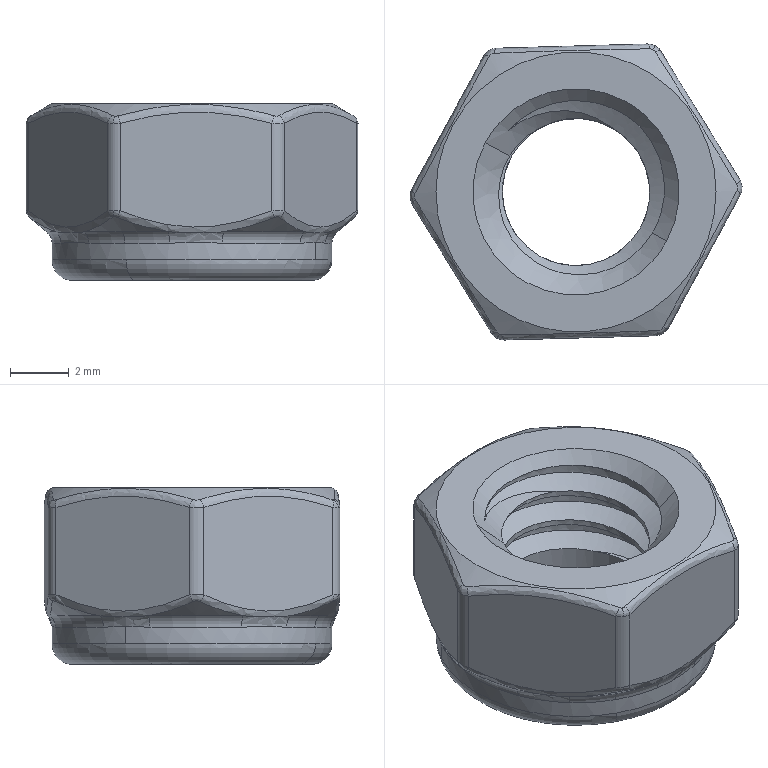Part | SolidWorks | features BaseBody 1 | 1 solid | 89 faces | box 11.269 x 10.041 x 6 mm | volume 327.548 mm3 | spline 37 | cylinder 22 | plane 10 | cone 10 | torus 10 | commonest cylinder face diameters 5 x9 1 x7 7 x3 9.5 x3